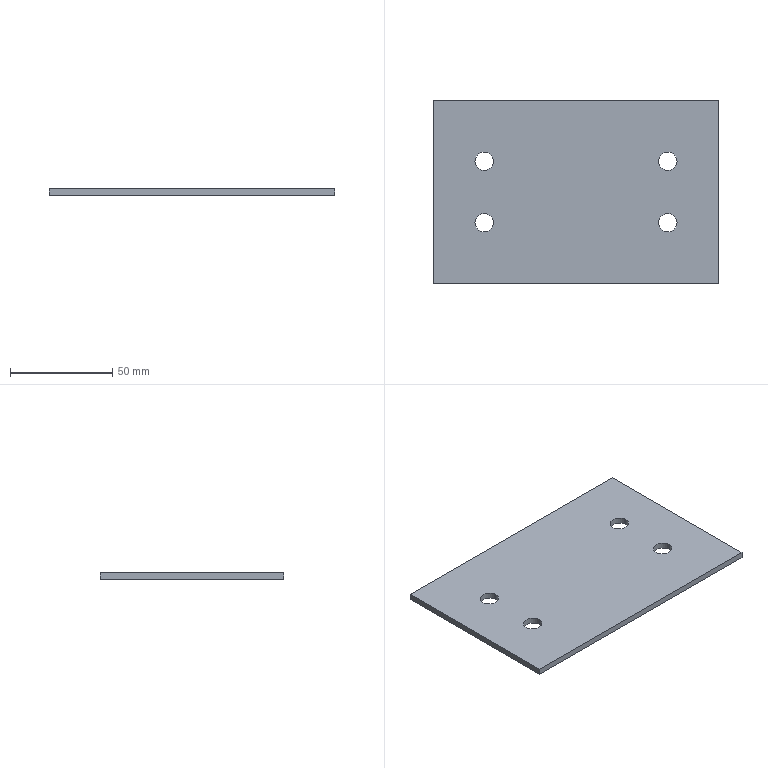Part | STEP file | Microwave Drying Flat Conveyor-CN2500x400-105-103 | 1 solid | 14 faces | box 140 x 90 x 3 mm | volume 37037 mm3 | cylinder 8 | plane 6 | commonest cylinder face diameters 9 x8
STEP:
#1=CARTESIAN_POINT('',(-49.5,-15.,3.));
#2=VERTEX_POINT('',#1);
#3=CARTESIAN_POINT('',(-40.5,-15.,3.));
#4=VERTEX_POINT('',#3);
#5=CARTESIAN_POINT('',(-45.,-15.,3.));
#6=DIRECTION('',(0.,0.,1.));
#7=DIRECTION('',(1.,0.,0.));
#8=AXIS2_PLACEMENT_3D('',#5,#6,#7);
#9=CIRCLE('',#8,4.5);
#10=EDGE_CURVE('',#2,#4,#9,.T.);
#11=ORIENTED_EDGE('',*,*,#10,.T.);
#12=CARTESIAN_POINT('',(-40.5,-15.,0.));
#13=VERTEX_POINT('',#12);
#14=CARTESIAN_POINT('',(-40.5,-15.,3.));
#15=DIRECTION('',(0.,0.,-1.));
#16=VECTOR('',#15,1000.);
#17=LINE('',#14,#16);
#18=EDGE_CURVE('',#4,#13,#17,.T.);
#19=ORIENTED_EDGE('',*,*,#18,.T.);
#20=CARTESIAN_POINT('',(-49.5,-15.,0.));
#21=VERTEX_POINT('',#20);
#22=CARTESIAN_POINT('',(-45.,-15.,0.));
#23=DIRECTION('',(0.,0.,1.));
#24=DIRECTION('',(1.,0.,0.));
#25=AXIS2_PLACEMENT_3D('',#22,#23,#24);
#26=CIRCLE('',#25,4.5);
#27=EDGE_CURVE('',#21,#13,#26,.T.);
#28=ORIENTED_EDGE('',*,*,#27,.F.);
#29=CARTESIAN_POINT('',(-49.5,-15.,3.));
#30=DIRECTION('',(0.,0.,-1.));
#31=VECTOR('',#30,1000.);
#32=LINE('',#29,#31);
#33=EDGE_CURVE('',#2,#21,#32,.T.);
#34=ORIENTED_EDGE('',*,*,#33,.F.);
#35=EDGE_LOOP('',(#11,#19,#28,#34));
#36=FACE_OUTER_BOUND('',#35,.T.);
#37=CARTESIAN_POINT('',(-45.,-15.,3.));
#38=DIRECTION('',(0.,0.,-1.));
#39=DIRECTION('',(-1.,0.,0.));
#40=AXIS2_PLACEMENT_3D('',#37,#38,#39);
#41=CYLINDRICAL_SURFACE('',#40,4.5);
#42=ADVANCED_FACE('',(#36),#41,.F.);
#43=CARTESIAN_POINT('',(40.5,-15.,3.));
#44=VERTEX_POINT('',#43);
#45=CARTESIAN_POINT('',(49.5,-15.,3.));
#46=VERTEX_POINT('',#45);
#47=CARTESIAN_POINT('',(45.,-15.,3.));
#48=DIRECTION('',(0.,0.,1.));
#49=DIRECTION('',(1.,0.,0.));
#50=AXIS2_PLACEMENT_3D('',#47,#48,#49);
#51=CIRCLE('',#50,4.5);
#52=EDGE_CURVE('',#44,#46,#51,.T.);
#53=ORIENTED_EDGE('',*,*,#52,.T.);
#54=CARTESIAN_POINT('',(49.5,-15.,0.));
#55=VERTEX_POINT('',#54);
#56=CARTESIAN_POINT('',(49.5,-15.,3.));
#57=DIRECTION('',(0.,0.,-1.));
#58=VECTOR('',#57,1000.);
#59=LINE('',#56,#58);
#60=EDGE_CURVE('',#46,#55,#59,.T.);
#61=ORIENTED_EDGE('',*,*,#60,.T.);
#62=CARTESIAN_POINT('',(40.5,-15.,0.));
#63=VERTEX_POINT('',#62);
#64=CARTESIAN_POINT('',(45.,-15.,0.));
#65=DIRECTION('',(0.,0.,1.));
#66=DIRECTION('',(1.,0.,0.));
#67=AXIS2_PLACEMENT_3D('',#64,#65,#66);
#68=CIRCLE('',#67,4.5);
#69=EDGE_CURVE('',#63,#55,#68,.T.);
#70=ORIENTED_EDGE('',*,*,#69,.F.);
#71=CARTESIAN_POINT('',(40.5,-15.,3.));
#72=DIRECTION('',(0.,0.,-1.));
#73=VECTOR('',#72,1000.);
#74=LINE('',#71,#73);
#75=EDGE_CURVE('',#44,#63,#74,.T.);
#76=ORIENTED_EDGE('',*,*,#75,.F.);
#77=EDGE_LOOP('',(#53,#61,#70,#76));
#78=FACE_OUTER_BOUND('',#77,.T.);
#79=CARTESIAN_POINT('',(45.,-15.,3.));
#80=DIRECTION('',(0.,0.,-1.));
#81=DIRECTION('',(-1.,0.,0.));
#82=AXIS2_PLACEMENT_3D('',#79,#80,#81);
#83=CYLINDRICAL_SURFACE('',#82,4.5);
#84=ADVANCED_FACE('',(#78),#83,.F.);
#85=CARTESIAN_POINT('',(40.5,15.,3.));
#86=VERTEX_POINT('',#85);
#87=CARTESIAN_POINT('',(49.5,15.,3.));
#88=VERTEX_POINT('',#87);
#89=CARTESIAN_POINT('',(45.,15.,3.));
#90=DIRECTION('',(0.,0.,1.));
#91=DIRECTION('',(1.,0.,0.));
#92=AXIS2_PLACEMENT_3D('',#89,#90,#91);
#93=CIRCLE('',#92,4.5);
#94=EDGE_CURVE('',#86,#88,#93,.T.);
#95=ORIENTED_EDGE('',*,*,#94,.T.);
#96=CARTESIAN_POINT('',(49.5,15.,0.));
#97=VERTEX_POINT('',#96);
#98=CARTESIAN_POINT('',(49.5,15.,3.));
#99=DIRECTION('',(0.,0.,-1.));
#100=VECTOR('',#99,1000.);
#101=LINE('',#98,#100);
#102=EDGE_CURVE('',#88,#97,#101,.T.);
#103=ORIENTED_EDGE('',*,*,#102,.T.);
#104=CARTESIAN_POINT('',(40.5,15.,0.));
#105=VERTEX_POINT('',#104);
#106=CARTESIAN_POINT('',(45.,15.,0.));
#107=DIRECTION('',(0.,0.,1.));
#108=DIRECTION('',(1.,0.,0.));
#109=AXIS2_PLACEMENT_3D('',#106,#107,#108);
#110=CIRCLE('',#109,4.5);
#111=EDGE_CURVE('',#105,#97,#110,.T.);
#112=ORIENTED_EDGE('',*,*,#111,.F.);
#113=CARTESIAN_POINT('',(40.5,15.,3.));
#114=DIRECTION('',(0.,0.,-1.));
#115=VECTOR('',#114,1000.);
#116=LINE('',#113,#115);
#117=EDGE_CURVE('',#86,#105,#116,.T.);
#118=ORIENTED_EDGE('',*,*,#117,.F.);
#119=EDGE_LOOP('',(#95,#103,#112,#118));
#120=FACE_OUTER_BOUND('',#119,.T.);
#121=CARTESIAN_POINT('',(45.,15.,3.));
#122=DIRECTION('',(0.,0.,-1.));
#123=DIRECTION('',(-1.,0.,0.));
#124=AXIS2_PLACEMENT_3D('',#121,#122,#123);
#125=CYLINDRICAL_SURFACE('',#124,4.5);
#126=ADVANCED_FACE('',(#120),#125,.F.);
#127=CARTESIAN_POINT('',(-49.5,15.,3.));
#128=VERTEX_POINT('',#127);
#129=CARTESIAN_POINT('',(-40.5,15.,3.));
#130=VERTEX_POINT('',#129);
#131=CARTESIAN_POINT('',(-45.,15.,3.));
#132=DIRECTION('',(0.,0.,1.));
#133=DIRECTION('',(1.,0.,0.));
#134=AXIS2_PLACEMENT_3D('',#131,#132,#133);
#135=CIRCLE('',#134,4.5);
#136=EDGE_CURVE('',#128,#130,#135,.T.);
#137=ORIENTED_EDGE('',*,*,#136,.T.);
#138=CARTESIAN_POINT('',(-40.5,15.,0.));
#139=VERTEX_POINT('',#138);
#140=CARTESIAN_POINT('',(-40.5,15.,3.));
#141=DIRECTION('',(0.,0.,-1.));
#142=VECTOR('',#141,1000.);
#143=LINE('',#140,#142);
#144=EDGE_CURVE('',#130,#139,#143,.T.);
#145=ORIENTED_EDGE('',*,*,#144,.T.);
#146=CARTESIAN_POINT('',(-49.5,15.,0.));
#147=VERTEX_POINT('',#146);
#148=CARTESIAN_POINT('',(-45.,15.,0.));
#149=DIRECTION('',(0.,0.,1.));
#150=DIRECTION('',(1.,0.,0.));
#151=AXIS2_PLACEMENT_3D('',#148,#149,#150);
#152=CIRCLE('',#151,4.5);
#153=EDGE_CURVE('',#147,#139,#152,.T.);
#154=ORIENTED_EDGE('',*,*,#153,.F.);
#155=CARTESIAN_POINT('',(-49.5,15.,3.));
#156=DIRECTION('',(0.,0.,-1.));
#157=VECTOR('',#156,1000.);
#158=LINE('',#155,#157);
#159=EDGE_CURVE('',#128,#147,#158,.T.);
#160=ORIENTED_EDGE('',*,*,#159,.F.);
#161=EDGE_LOOP('',(#137,#145,#154,#160));
#162=FACE_OUTER_BOUND('',#161,.T.);
#163=CARTESIAN_POINT('',(-45.,15.,3.));
#164=DIRECTION('',(0.,0.,-1.));
#165=DIRECTION('',(-1.,0.,0.));
#166=AXIS2_PLACEMENT_3D('',#163,#164,#165);
#167=CYLINDRICAL_SURFACE('',#166,4.5);
#168=ADVANCED_FACE('',(#162),#167,.F.);
#169=ORIENTED_EDGE('',*,*,#52,.F.);
#170=CARTESIAN_POINT('',(45.,-15.,3.));
#171=DIRECTION('',(0.,0.,1.));
#172=DIRECTION('',(1.,0.,0.));
#173=AXIS2_PLACEMENT_3D('',#170,#171,#172);
#174=CIRCLE('',#173,4.5);
#175=EDGE_CURVE('',#46,#44,#174,.T.);
#176=ORIENTED_EDGE('',*,*,#175,.F.);
#177=EDGE_LOOP('',(#169,#176));
#178=FACE_BOUND('',#177,.T.);
#179=ORIENTED_EDGE('',*,*,#136,.F.);
#180=CARTESIAN_POINT('',(-45.,15.,3.));
#181=DIRECTION('',(0.,0.,1.));
#182=DIRECTION('',(1.,0.,0.));
#183=AXIS2_PLACEMENT_3D('',#180,#181,#182);
#184=CIRCLE('',#183,4.5);
#185=EDGE_CURVE('',#130,#128,#184,.T.);
#186=ORIENTED_EDGE('',*,*,#185,.F.);
#187=EDGE_LOOP('',(#179,#186));
#188=FACE_BOUND('',#187,.T.);
#189=CARTESIAN_POINT('',(70.,-45.,3.));
#190=VERTEX_POINT('',#189);
#191=CARTESIAN_POINT('',(70.,45.,3.));
#192=VERTEX_POINT('',#191);
#193=CARTESIAN_POINT('',(70.,45.,3.));
#194=DIRECTION('',(0.,1.,0.));
#195=VECTOR('',#194,1000.);
#196=LINE('',#193,#195);
#197=EDGE_CURVE('',#190,#192,#196,.T.);
#198=ORIENTED_EDGE('',*,*,#197,.T.);
#199=CARTESIAN_POINT('',(-70.,45.,3.));
#200=VERTEX_POINT('',#199);
#201=CARTESIAN_POINT('',(-70.,45.,3.));
#202=DIRECTION('',(-1.,0.,0.));
#203=VECTOR('',#202,1000.);
#204=LINE('',#201,#203);
#205=EDGE_CURVE('',#192,#200,#204,.T.);
#206=ORIENTED_EDGE('',*,*,#205,.T.);
#207=CARTESIAN_POINT('',(-70.,-45.,3.));
#208=VERTEX_POINT('',#207);
#209=CARTESIAN_POINT('',(-70.,45.,3.));
#210=DIRECTION('',(0.,-1.,0.));
#211=VECTOR('',#210,1000.);
#212=LINE('',#209,#211);
#213=EDGE_CURVE('',#200,#208,#212,.T.);
#214=ORIENTED_EDGE('',*,*,#213,.T.);
#215=CARTESIAN_POINT('',(-70.,-45.,3.));
#216=DIRECTION('',(1.,0.,0.));
#217=VECTOR('',#216,1000.);
#218=LINE('',#215,#217);
#219=EDGE_CURVE('',#208,#190,#218,.T.);
#220=ORIENTED_EDGE('',*,*,#219,.T.);
#221=EDGE_LOOP('',(#198,#206,#214,#220));
#222=FACE_OUTER_BOUND('',#221,.T.);
#223=ORIENTED_EDGE('',*,*,#94,.F.);
#224=CARTESIAN_POINT('',(45.,15.,3.));
#225=DIRECTION('',(0.,0.,1.));
#226=DIRECTION('',(1.,0.,0.));
#227=AXIS2_PLACEMENT_3D('',#224,#225,#226);
#228=CIRCLE('',#227,4.5);
#229=EDGE_CURVE('',#88,#86,#228,.T.);
#230=ORIENTED_EDGE('',*,*,#229,.F.);
#231=EDGE_LOOP('',(#223,#230));
#232=FACE_BOUND('',#231,.T.);
#233=ORIENTED_EDGE('',*,*,#10,.F.);
#234=CARTESIAN_POINT('',(-45.,-15.,3.));
#235=DIRECTION('',(0.,0.,1.));
#236=DIRECTION('',(1.,0.,0.));
#237=AXIS2_PLACEMENT_3D('',#234,#235,#236);
#238=CIRCLE('',#237,4.5);
#239=EDGE_CURVE('',#4,#2,#238,.T.);
#240=ORIENTED_EDGE('',*,*,#239,.F.);
#241=EDGE_LOOP('',(#233,#240));
#242=FACE_BOUND('',#241,.T.);
#243=CARTESIAN_POINT('',(0.,0.,3.));
#244=DIRECTION('',(0.,0.,1.));
#245=DIRECTION('',(1.,0.,0.));
#246=AXIS2_PLACEMENT_3D('',#243,#244,#245);
#247=PLANE('',#246);
#248=ADVANCED_FACE('',(#178,#188,#222,#232,#242),#247,.T.);
#249=CARTESIAN_POINT('',(70.,-45.,0.));
#250=VERTEX_POINT('',#249);
#251=CARTESIAN_POINT('',(70.,45.,0.));
#252=VERTEX_POINT('',#251);
#253=CARTESIAN_POINT('',(70.,45.,0.));
#254=DIRECTION('',(0.,1.,0.));
#255=VECTOR('',#254,1000.);
#256=LINE('',#253,#255);
#257=EDGE_CURVE('',#250,#252,#256,.T.);
#258=ORIENTED_EDGE('',*,*,#257,.F.);
#259=CARTESIAN_POINT('',(-70.,-45.,0.));
#260=VERTEX_POINT('',#259);
#261=CARTESIAN_POINT('',(-70.,-45.,0.));
#262=DIRECTION('',(1.,0.,0.));
#263=VECTOR('',#262,1000.);
#264=LINE('',#261,#263);
#265=EDGE_CURVE('',#260,#250,#264,.T.);
#266=ORIENTED_EDGE('',*,*,#265,.F.);
#267=CARTESIAN_POINT('',(-70.,45.,0.));
#268=VERTEX_POINT('',#267);
#269=CARTESIAN_POINT('',(-70.,45.,0.));
#270=DIRECTION('',(0.,-1.,0.));
#271=VECTOR('',#270,1000.);
#272=LINE('',#269,#271);
#273=EDGE_CURVE('',#268,#260,#272,.T.);
#274=ORIENTED_EDGE('',*,*,#273,.F.);
#275=CARTESIAN_POINT('',(-70.,45.,0.));
#276=DIRECTION('',(-1.,0.,0.));
#277=VECTOR('',#276,1000.);
#278=LINE('',#275,#277);
#279=EDGE_CURVE('',#252,#268,#278,.T.);
#280=ORIENTED_EDGE('',*,*,#279,.F.);
#281=EDGE_LOOP('',(#258,#266,#274,#280));
#282=FACE_OUTER_BOUND('',#281,.T.);
#283=ORIENTED_EDGE('',*,*,#153,.T.);
#284=CARTESIAN_POINT('',(-45.,15.,0.));
#285=DIRECTION('',(0.,0.,1.));
#286=DIRECTION('',(1.,0.,0.));
#287=AXIS2_PLACEMENT_3D('',#284,#285,#286);
#288=CIRCLE('',#287,4.5);
#289=EDGE_CURVE('',#139,#147,#288,.T.);
#290=ORIENTED_EDGE('',*,*,#289,.T.);
#291=EDGE_LOOP('',(#283,#290));
#292=FACE_BOUND('',#291,.T.);
#293=ORIENTED_EDGE('',*,*,#111,.T.);
#294=CARTESIAN_POINT('',(45.,15.,0.));
#295=DIRECTION('',(0.,0.,1.));
#296=DIRECTION('',(1.,0.,0.));
#297=AXIS2_PLACEMENT_3D('',#294,#295,#296);
#298=CIRCLE('',#297,4.5);
#299=EDGE_CURVE('',#97,#105,#298,.T.);
#300=ORIENTED_EDGE('',*,*,#299,.T.);
#301=EDGE_LOOP('',(#293,#300));
#302=FACE_BOUND('',#301,.T.);
#303=ORIENTED_EDGE('',*,*,#69,.T.);
#304=CARTESIAN_POINT('',(45.,-15.,0.));
#305=DIRECTION('',(0.,0.,1.));
#306=DIRECTION('',(1.,0.,0.));
#307=AXIS2_PLACEMENT_3D('',#304,#305,#306);
#308=CIRCLE('',#307,4.5);
#309=EDGE_CURVE('',#55,#63,#308,.T.);
#310=ORIENTED_EDGE('',*,*,#309,.T.);
#311=EDGE_LOOP('',(#303,#310));
#312=FACE_BOUND('',#311,.T.);
#313=ORIENTED_EDGE('',*,*,#27,.T.);
#314=CARTESIAN_POINT('',(-45.,-15.,0.));
#315=DIRECTION('',(0.,0.,1.));
#316=DIRECTION('',(1.,0.,0.));
#317=AXIS2_PLACEMENT_3D('',#314,#315,#316);
#318=CIRCLE('',#317,4.5);
#319=EDGE_CURVE('',#13,#21,#318,.T.);
#320=ORIENTED_EDGE('',*,*,#319,.T.);
#321=EDGE_LOOP('',(#313,#320));
#322=FACE_BOUND('',#321,.T.);
#323=CARTESIAN_POINT('',(0.,0.,0.));
#324=DIRECTION('',(0.,0.,1.));
#325=DIRECTION('',(1.,0.,0.));
#326=AXIS2_PLACEMENT_3D('',#323,#324,#325);
#327=PLANE('',#326);
#328=ADVANCED_FACE('',(#282,#292,#302,#312,#322),#327,.F.);
#329=ORIENTED_EDGE('',*,*,#257,.T.);
#330=CARTESIAN_POINT('',(70.,45.,3.));
#331=DIRECTION('',(0.,0.,-1.));
#332=VECTOR('',#331,1000.);
#333=LINE('',#330,#332);
#334=EDGE_CURVE('',#192,#252,#333,.T.);
#335=ORIENTED_EDGE('',*,*,#334,.F.);
#336=ORIENTED_EDGE('',*,*,#197,.F.);
#337=CARTESIAN_POINT('',(70.,-45.,3.));
#338=DIRECTION('',(0.,0.,-1.));
#339=VECTOR('',#338,1000.);
#340=LINE('',#337,#339);
#341=EDGE_CURVE('',#190,#250,#340,.T.);
#342=ORIENTED_EDGE('',*,*,#341,.T.);
#343=EDGE_LOOP('',(#329,#335,#336,#342));
#344=FACE_OUTER_BOUND('',#343,.T.);
#345=CARTESIAN_POINT('',(70.,45.,3.));
#346=DIRECTION('',(-1.,0.,0.));
#347=DIRECTION('',(0.,-1.,0.));
#348=AXIS2_PLACEMENT_3D('',#345,#346,#347);
#349=PLANE('',#348);
#350=ADVANCED_FACE('',(#344),#349,.F.);
#351=ORIENTED_EDGE('',*,*,#279,.T.);
#352=CARTESIAN_POINT('',(-70.,45.,3.));
#353=DIRECTION('',(0.,0.,-1.));
#354=VECTOR('',#353,1000.);
#355=LINE('',#352,#354);
#356=EDGE_CURVE('',#200,#268,#355,.T.);
#357=ORIENTED_EDGE('',*,*,#356,.F.);
#358=ORIENTED_EDGE('',*,*,#205,.F.);
#359=ORIENTED_EDGE('',*,*,#334,.T.);
#360=EDGE_LOOP('',(#351,#357,#358,#359));
#361=FACE_OUTER_BOUND('',#360,.T.);
#362=CARTESIAN_POINT('',(-70.,45.,3.));
#363=DIRECTION('',(0.,-1.,0.));
#364=DIRECTION('',(0.,0.,-1.));
#365=AXIS2_PLACEMENT_3D('',#362,#363,#364);
#366=PLANE('',#365);
#367=ADVANCED_FACE('',(#361),#366,.F.);
#368=ORIENTED_EDGE('',*,*,#273,.T.);
#369=CARTESIAN_POINT('',(-70.,-45.,3.));
#370=DIRECTION('',(0.,0.,-1.));
#371=VECTOR('',#370,1000.);
#372=LINE('',#369,#371);
#373=EDGE_CURVE('',#208,#260,#372,.T.);
#374=ORIENTED_EDGE('',*,*,#373,.F.);
#375=ORIENTED_EDGE('',*,*,#213,.F.);
#376=ORIENTED_EDGE('',*,*,#356,.T.);
#377=EDGE_LOOP('',(#368,#374,#375,#376));
#378=FACE_OUTER_BOUND('',#377,.T.);
#379=CARTESIAN_POINT('',(-70.,45.,3.));
#380=DIRECTION('',(1.,0.,0.));
#381=DIRECTION('',(0.,1.,0.));
#382=AXIS2_PLACEMENT_3D('',#379,#380,#381);
#383=PLANE('',#382);
#384=ADVANCED_FACE('',(#378),#383,.F.);
#385=ORIENTED_EDGE('',*,*,#265,.T.);
#386=ORIENTED_EDGE('',*,*,#341,.F.);
#387=ORIENTED_EDGE('',*,*,#219,.F.);
#388=ORIENTED_EDGE('',*,*,#373,.T.);
#389=EDGE_LOOP('',(#385,#386,#387,#388));
#390=FACE_OUTER_BOUND('',#389,.T.);
#391=CARTESIAN_POINT('',(-70.,-45.,3.));
#392=DIRECTION('',(0.,1.,0.));
#393=DIRECTION('',(0.,0.,1.));
#394=AXIS2_PLACEMENT_3D('',#391,#392,#393);
#395=PLANE('',#394);
#396=ADVANCED_FACE('',(#390),#395,.F.);
#397=ORIENTED_EDGE('',*,*,#144,.F.);
#398=ORIENTED_EDGE('',*,*,#185,.T.);
#399=ORIENTED_EDGE('',*,*,#159,.T.);
#400=ORIENTED_EDGE('',*,*,#289,.F.);
#401=EDGE_LOOP('',(#397,#398,#399,#400));
#402=FACE_OUTER_BOUND('',#401,.T.);
#403=CARTESIAN_POINT('',(-45.,15.,3.));
#404=DIRECTION('',(0.,0.,-1.));
#405=DIRECTION('',(-1.,0.,0.));
#406=AXIS2_PLACEMENT_3D('',#403,#404,#405);
#407=CYLINDRICAL_SURFACE('',#406,4.5);
#408=ADVANCED_FACE('',(#402),#407,.F.);
#409=ORIENTED_EDGE('',*,*,#102,.F.);
#410=ORIENTED_EDGE('',*,*,#229,.T.);
#411=ORIENTED_EDGE('',*,*,#117,.T.);
#412=ORIENTED_EDGE('',*,*,#299,.F.);
#413=EDGE_LOOP('',(#409,#410,#411,#412));
#414=FACE_OUTER_BOUND('',#413,.T.);
#415=CARTESIAN_POINT('',(45.,15.,3.));
#416=DIRECTION('',(0.,0.,-1.));
#417=DIRECTION('',(-1.,0.,0.));
#418=AXIS2_PLACEMENT_3D('',#415,#416,#417);
#419=CYLINDRICAL_SURFACE('',#418,4.5);
#420=ADVANCED_FACE('',(#414),#419,.F.);
#421=ORIENTED_EDGE('',*,*,#60,.F.);
#422=ORIENTED_EDGE('',*,*,#175,.T.);
#423=ORIENTED_EDGE('',*,*,#75,.T.);
#424=ORIENTED_EDGE('',*,*,#309,.F.);
#425=EDGE_LOOP('',(#421,#422,#423,#424));
#426=FACE_OUTER_BOUND('',#425,.T.);
#427=CARTESIAN_POINT('',(45.,-15.,3.));
#428=DIRECTION('',(0.,0.,-1.));
#429=DIRECTION('',(-1.,0.,0.));
#430=AXIS2_PLACEMENT_3D('',#427,#428,#429);
#431=CYLINDRICAL_SURFACE('',#430,4.5);
#432=ADVANCED_FACE('',(#426),#431,.F.);
#433=ORIENTED_EDGE('',*,*,#18,.F.);
#434=ORIENTED_EDGE('',*,*,#239,.T.);
#435=ORIENTED_EDGE('',*,*,#33,.T.);
#436=ORIENTED_EDGE('',*,*,#319,.F.);
#437=EDGE_LOOP('',(#433,#434,#435,#436));
#438=FACE_OUTER_BOUND('',#437,.T.);
#439=CARTESIAN_POINT('',(-45.,-15.,3.));
#440=DIRECTION('',(0.,0.,-1.));
#441=DIRECTION('',(-1.,0.,0.));
#442=AXIS2_PLACEMENT_3D('',#439,#440,#441);
#443=CYLINDRICAL_SURFACE('',#442,4.5);
#444=ADVANCED_FACE('',(#438),#443,.F.);
#445=CLOSED_SHELL('',(#42,#84,#126,#168,#248,#328,#350,#367,#384,#396,#408,#420,#432,#444));
#446=MANIFOLD_SOLID_BREP('',#445);
#447=CARTESIAN_POINT('',(0.,0.,0.));
#448=DIRECTION('',(0.,0.,1.));
#449=DIRECTION('',(1.,0.,0.));
#450=AXIS2_PLACEMENT_3D('',#447,#448,#449);
#451=(LENGTH_UNIT()NAMED_UNIT(*)SI_UNIT(.MILLI.,.METRE.));
#452=UNCERTAINTY_MEASURE_WITH_UNIT(LENGTH_MEASURE(0.00001),#451,'','');
#453=(NAMED_UNIT(*)PLANE_ANGLE_UNIT()SI_UNIT($,.RADIAN.));
#454=(NAMED_UNIT(*)SI_UNIT($,.STERADIAN.)SOLID_ANGLE_UNIT());
#455=(GEOMETRIC_REPRESENTATION_CONTEXT(3)GLOBAL_UNCERTAINTY_ASSIGNED_CONTEXT((#452))GLOBAL_UNIT_ASSIGNED_CONTEXT((#451,#453,#454))REPRESENTATION_CONTEXT('',''));
#456=ADVANCED_BREP_SHAPE_REPRESENTATION('',(#446,#450),#455);